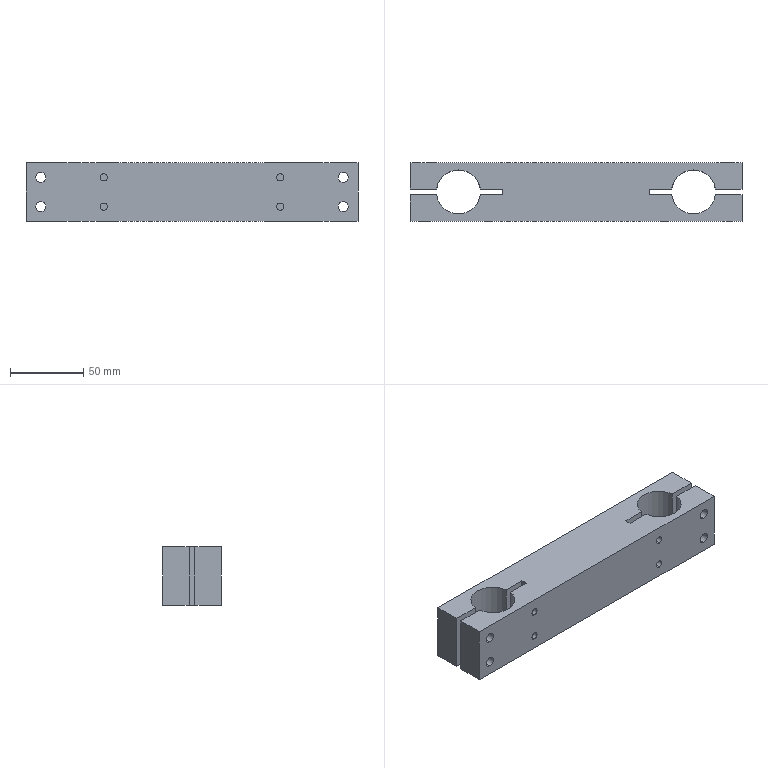Part | STEP file | 2004 Support shaft connecting plate A | 1 solid | 58 faces | box 226 x 40 x 40 mm | volume 281782 mm3 | cylinder 36 | plane 22 | commonest cylinder face diameters 5 x8 6.8 x8 9 x8 15 x8 30 x4